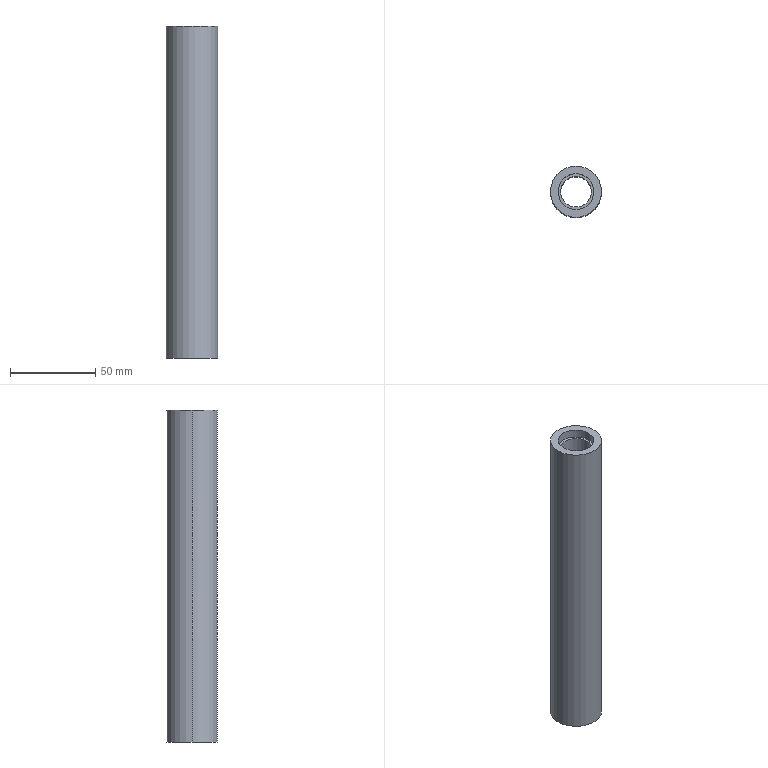Part | STEP file | MT-COMBO-119-S042 | 1 solid | 12 faces | box 30 x 30 x 195 mm | volume 87297 mm3 | cylinder 8 | plane 4 | commonest cylinder face diameters 21 x4 18 x2 30 x2
STEP:
#1=CARTESIAN_POINT('',(-9.,0.,190.));
#2=VERTEX_POINT('',#1);
#3=CARTESIAN_POINT('',(9.,0.,190.));
#4=VERTEX_POINT('',#3);
#5=CARTESIAN_POINT('',(0.,0.,190.));
#6=DIRECTION('',(0.,0.,1.));
#7=DIRECTION('',(1.,0.,0.));
#8=AXIS2_PLACEMENT_3D('',#5,#6,#7);
#9=CIRCLE('',#8,9.);
#10=EDGE_CURVE('',#2,#4,#9,.T.);
#11=ORIENTED_EDGE('',*,*,#10,.T.);
#12=CARTESIAN_POINT('',(9.,0.,5.));
#13=VERTEX_POINT('',#12);
#14=CARTESIAN_POINT('',(9.,0.,195.));
#15=DIRECTION('',(0.,0.,-1.));
#16=VECTOR('',#15,1000.);
#17=LINE('',#14,#16);
#18=EDGE_CURVE('',#4,#13,#17,.T.);
#19=ORIENTED_EDGE('',*,*,#18,.T.);
#20=CARTESIAN_POINT('',(-9.,0.,5.));
#21=VERTEX_POINT('',#20);
#22=CARTESIAN_POINT('',(0.,0.,5.));
#23=DIRECTION('',(0.,0.,-1.));
#24=DIRECTION('',(-1.,0.,0.));
#25=AXIS2_PLACEMENT_3D('',#22,#23,#24);
#26=CIRCLE('',#25,9.);
#27=EDGE_CURVE('',#13,#21,#26,.T.);
#28=ORIENTED_EDGE('',*,*,#27,.T.);
#29=CARTESIAN_POINT('',(-9.,0.,195.));
#30=DIRECTION('',(0.,0.,-1.));
#31=VECTOR('',#30,1000.);
#32=LINE('',#29,#31);
#33=EDGE_CURVE('',#2,#21,#32,.T.);
#34=ORIENTED_EDGE('',*,*,#33,.F.);
#35=EDGE_LOOP('',(#11,#19,#28,#34));
#36=FACE_OUTER_BOUND('',#35,.T.);
#37=CARTESIAN_POINT('',(0.,0.,195.));
#38=DIRECTION('',(0.,0.,-1.));
#39=DIRECTION('',(-1.,0.,0.));
#40=AXIS2_PLACEMENT_3D('',#37,#38,#39);
#41=CYLINDRICAL_SURFACE('',#40,9.);
#42=ADVANCED_FACE('',(#36),#41,.F.);
#43=CARTESIAN_POINT('',(10.5,0.,5.));
#44=VERTEX_POINT('',#43);
#45=CARTESIAN_POINT('',(-10.5,0.,5.));
#46=VERTEX_POINT('',#45);
#47=CARTESIAN_POINT('',(0.,0.,5.));
#48=DIRECTION('',(0.,0.,-1.));
#49=DIRECTION('',(-1.,0.,0.));
#50=AXIS2_PLACEMENT_3D('',#47,#48,#49);
#51=CIRCLE('',#50,10.5);
#52=EDGE_CURVE('',#44,#46,#51,.T.);
#53=ORIENTED_EDGE('',*,*,#52,.F.);
#54=CARTESIAN_POINT('',(10.5,0.,0.));
#55=VERTEX_POINT('',#54);
#56=CARTESIAN_POINT('',(10.5,0.,5.));
#57=DIRECTION('',(0.,0.,-1.));
#58=VECTOR('',#57,1000.);
#59=LINE('',#56,#58);
#60=EDGE_CURVE('',#44,#55,#59,.T.);
#61=ORIENTED_EDGE('',*,*,#60,.T.);
#62=CARTESIAN_POINT('',(-10.5,0.,0.));
#63=VERTEX_POINT('',#62);
#64=CARTESIAN_POINT('',(0.,0.,0.));
#65=DIRECTION('',(0.,0.,-1.));
#66=DIRECTION('',(-1.,0.,0.));
#67=AXIS2_PLACEMENT_3D('',#64,#65,#66);
#68=CIRCLE('',#67,10.5);
#69=EDGE_CURVE('',#55,#63,#68,.T.);
#70=ORIENTED_EDGE('',*,*,#69,.T.);
#71=CARTESIAN_POINT('',(-10.5,0.,5.));
#72=DIRECTION('',(0.,0.,-1.));
#73=VECTOR('',#72,1000.);
#74=LINE('',#71,#73);
#75=EDGE_CURVE('',#46,#63,#74,.T.);
#76=ORIENTED_EDGE('',*,*,#75,.F.);
#77=EDGE_LOOP('',(#53,#61,#70,#76));
#78=FACE_OUTER_BOUND('',#77,.T.);
#79=CARTESIAN_POINT('',(0.,0.,5.));
#80=DIRECTION('',(0.,0.,-1.));
#81=DIRECTION('',(-1.,0.,0.));
#82=AXIS2_PLACEMENT_3D('',#79,#80,#81);
#83=CYLINDRICAL_SURFACE('',#82,10.5);
#84=ADVANCED_FACE('',(#78),#83,.F.);
#85=CARTESIAN_POINT('',(-10.5,0.,190.));
#86=VERTEX_POINT('',#85);
#87=CARTESIAN_POINT('',(10.5,0.,190.));
#88=VERTEX_POINT('',#87);
#89=CARTESIAN_POINT('',(0.,0.,190.));
#90=DIRECTION('',(0.,0.,1.));
#91=DIRECTION('',(1.,0.,0.));
#92=AXIS2_PLACEMENT_3D('',#89,#90,#91);
#93=CIRCLE('',#92,10.5);
#94=EDGE_CURVE('',#86,#88,#93,.T.);
#95=ORIENTED_EDGE('',*,*,#94,.F.);
#96=CARTESIAN_POINT('',(-10.5,0.,195.));
#97=VERTEX_POINT('',#96);
#98=CARTESIAN_POINT('',(-10.5,0.,190.));
#99=DIRECTION('',(0.,0.,1.));
#100=VECTOR('',#99,1000.);
#101=LINE('',#98,#100);
#102=EDGE_CURVE('',#86,#97,#101,.T.);
#103=ORIENTED_EDGE('',*,*,#102,.T.);
#104=CARTESIAN_POINT('',(10.5,0.,195.));
#105=VERTEX_POINT('',#104);
#106=CARTESIAN_POINT('',(0.,0.,195.));
#107=DIRECTION('',(0.,0.,1.));
#108=DIRECTION('',(1.,0.,0.));
#109=AXIS2_PLACEMENT_3D('',#106,#107,#108);
#110=CIRCLE('',#109,10.5);
#111=EDGE_CURVE('',#97,#105,#110,.T.);
#112=ORIENTED_EDGE('',*,*,#111,.T.);
#113=CARTESIAN_POINT('',(10.5,0.,190.));
#114=DIRECTION('',(0.,0.,1.));
#115=VECTOR('',#114,1000.);
#116=LINE('',#113,#115);
#117=EDGE_CURVE('',#88,#105,#116,.T.);
#118=ORIENTED_EDGE('',*,*,#117,.F.);
#119=EDGE_LOOP('',(#95,#103,#112,#118));
#120=FACE_OUTER_BOUND('',#119,.T.);
#121=CARTESIAN_POINT('',(0.,0.,190.));
#122=DIRECTION('',(0.,0.,1.));
#123=DIRECTION('',(1.,0.,0.));
#124=AXIS2_PLACEMENT_3D('',#121,#122,#123);
#125=CYLINDRICAL_SURFACE('',#124,10.5);
#126=ADVANCED_FACE('',(#120),#125,.F.);
#127=CARTESIAN_POINT('',(15.,0.,195.));
#128=VERTEX_POINT('',#127);
#129=CARTESIAN_POINT('',(-15.,0.,195.));
#130=VERTEX_POINT('',#129);
#131=CARTESIAN_POINT('',(0.,0.,195.));
#132=DIRECTION('',(0.,0.,1.));
#133=DIRECTION('',(1.,0.,0.));
#134=AXIS2_PLACEMENT_3D('',#131,#132,#133);
#135=CIRCLE('',#134,15.);
#136=EDGE_CURVE('',#128,#130,#135,.T.);
#137=ORIENTED_EDGE('',*,*,#136,.F.);
#138=CARTESIAN_POINT('',(15.,0.,0.));
#139=VERTEX_POINT('',#138);
#140=CARTESIAN_POINT('',(15.,0.,195.));
#141=DIRECTION('',(0.,0.,-1.));
#142=VECTOR('',#141,1000.);
#143=LINE('',#140,#142);
#144=EDGE_CURVE('',#128,#139,#143,.T.);
#145=ORIENTED_EDGE('',*,*,#144,.T.);
#146=CARTESIAN_POINT('',(-15.,0.,0.));
#147=VERTEX_POINT('',#146);
#148=CARTESIAN_POINT('',(0.,0.,0.));
#149=DIRECTION('',(0.,0.,1.));
#150=DIRECTION('',(1.,0.,0.));
#151=AXIS2_PLACEMENT_3D('',#148,#149,#150);
#152=CIRCLE('',#151,15.);
#153=EDGE_CURVE('',#139,#147,#152,.T.);
#154=ORIENTED_EDGE('',*,*,#153,.T.);
#155=CARTESIAN_POINT('',(-15.,0.,195.));
#156=DIRECTION('',(0.,0.,-1.));
#157=VECTOR('',#156,1000.);
#158=LINE('',#155,#157);
#159=EDGE_CURVE('',#130,#147,#158,.T.);
#160=ORIENTED_EDGE('',*,*,#159,.F.);
#161=EDGE_LOOP('',(#137,#145,#154,#160));
#162=FACE_OUTER_BOUND('',#161,.T.);
#163=CARTESIAN_POINT('',(0.,0.,195.));
#164=DIRECTION('',(0.,0.,-1.));
#165=DIRECTION('',(-1.,0.,0.));
#166=AXIS2_PLACEMENT_3D('',#163,#164,#165);
#167=CYLINDRICAL_SURFACE('',#166,15.);
#168=ADVANCED_FACE('',(#162),#167,.T.);
#169=ORIENTED_EDGE('',*,*,#144,.F.);
#170=CARTESIAN_POINT('',(0.,0.,195.));
#171=DIRECTION('',(0.,0.,1.));
#172=DIRECTION('',(1.,0.,0.));
#173=AXIS2_PLACEMENT_3D('',#170,#171,#172);
#174=CIRCLE('',#173,15.);
#175=EDGE_CURVE('',#130,#128,#174,.T.);
#176=ORIENTED_EDGE('',*,*,#175,.F.);
#177=ORIENTED_EDGE('',*,*,#159,.T.);
#178=CARTESIAN_POINT('',(0.,0.,0.));
#179=DIRECTION('',(0.,0.,1.));
#180=DIRECTION('',(1.,0.,0.));
#181=AXIS2_PLACEMENT_3D('',#178,#179,#180);
#182=CIRCLE('',#181,15.);
#183=EDGE_CURVE('',#147,#139,#182,.T.);
#184=ORIENTED_EDGE('',*,*,#183,.T.);
#185=EDGE_LOOP('',(#169,#176,#177,#184));
#186=FACE_OUTER_BOUND('',#185,.T.);
#187=CARTESIAN_POINT('',(0.,0.,195.));
#188=DIRECTION('',(0.,0.,-1.));
#189=DIRECTION('',(-1.,0.,0.));
#190=AXIS2_PLACEMENT_3D('',#187,#188,#189);
#191=CYLINDRICAL_SURFACE('',#190,15.);
#192=ADVANCED_FACE('',(#186),#191,.T.);
#193=CARTESIAN_POINT('',(0.,0.,195.));
#194=DIRECTION('',(0.,0.,1.));
#195=DIRECTION('',(1.,0.,0.));
#196=AXIS2_PLACEMENT_3D('',#193,#194,#195);
#197=CIRCLE('',#196,10.5);
#198=EDGE_CURVE('',#105,#97,#197,.T.);
#199=ORIENTED_EDGE('',*,*,#198,.F.);
#200=ORIENTED_EDGE('',*,*,#111,.F.);
#201=EDGE_LOOP('',(#199,#200));
#202=FACE_BOUND('',#201,.T.);
#203=ORIENTED_EDGE('',*,*,#175,.T.);
#204=ORIENTED_EDGE('',*,*,#136,.T.);
#205=EDGE_LOOP('',(#203,#204));
#206=FACE_OUTER_BOUND('',#205,.T.);
#207=CARTESIAN_POINT('',(0.,0.,195.));
#208=DIRECTION('',(0.,0.,1.));
#209=DIRECTION('',(1.,0.,0.));
#210=AXIS2_PLACEMENT_3D('',#207,#208,#209);
#211=PLANE('',#210);
#212=ADVANCED_FACE('',(#202,#206),#211,.T.);
#213=CARTESIAN_POINT('',(0.,0.,0.));
#214=DIRECTION('',(0.,0.,-1.));
#215=DIRECTION('',(-1.,0.,0.));
#216=AXIS2_PLACEMENT_3D('',#213,#214,#215);
#217=CIRCLE('',#216,10.5);
#218=EDGE_CURVE('',#63,#55,#217,.T.);
#219=ORIENTED_EDGE('',*,*,#218,.F.);
#220=ORIENTED_EDGE('',*,*,#69,.F.);
#221=EDGE_LOOP('',(#219,#220));
#222=FACE_BOUND('',#221,.T.);
#223=ORIENTED_EDGE('',*,*,#183,.F.);
#224=ORIENTED_EDGE('',*,*,#153,.F.);
#225=EDGE_LOOP('',(#223,#224));
#226=FACE_OUTER_BOUND('',#225,.T.);
#227=CARTESIAN_POINT('',(0.,0.,0.));
#228=DIRECTION('',(0.,0.,1.));
#229=DIRECTION('',(1.,0.,0.));
#230=AXIS2_PLACEMENT_3D('',#227,#228,#229);
#231=PLANE('',#230);
#232=ADVANCED_FACE('',(#222,#226),#231,.F.);
#233=ORIENTED_EDGE('',*,*,#102,.F.);
#234=CARTESIAN_POINT('',(0.,0.,190.));
#235=DIRECTION('',(0.,0.,1.));
#236=DIRECTION('',(1.,0.,0.));
#237=AXIS2_PLACEMENT_3D('',#234,#235,#236);
#238=CIRCLE('',#237,10.5);
#239=EDGE_CURVE('',#88,#86,#238,.T.);
#240=ORIENTED_EDGE('',*,*,#239,.F.);
#241=ORIENTED_EDGE('',*,*,#117,.T.);
#242=ORIENTED_EDGE('',*,*,#198,.T.);
#243=EDGE_LOOP('',(#233,#240,#241,#242));
#244=FACE_OUTER_BOUND('',#243,.T.);
#245=CARTESIAN_POINT('',(0.,0.,190.));
#246=DIRECTION('',(0.,0.,1.));
#247=DIRECTION('',(1.,0.,0.));
#248=AXIS2_PLACEMENT_3D('',#245,#246,#247);
#249=CYLINDRICAL_SURFACE('',#248,10.5);
#250=ADVANCED_FACE('',(#244),#249,.F.);
#251=ORIENTED_EDGE('',*,*,#10,.F.);
#252=CARTESIAN_POINT('',(0.,0.,190.));
#253=DIRECTION('',(0.,0.,1.));
#254=DIRECTION('',(1.,0.,0.));
#255=AXIS2_PLACEMENT_3D('',#252,#253,#254);
#256=CIRCLE('',#255,9.);
#257=EDGE_CURVE('',#4,#2,#256,.T.);
#258=ORIENTED_EDGE('',*,*,#257,.F.);
#259=EDGE_LOOP('',(#251,#258));
#260=FACE_BOUND('',#259,.T.);
#261=ORIENTED_EDGE('',*,*,#239,.T.);
#262=ORIENTED_EDGE('',*,*,#94,.T.);
#263=EDGE_LOOP('',(#261,#262));
#264=FACE_OUTER_BOUND('',#263,.T.);
#265=CARTESIAN_POINT('',(0.,0.,190.));
#266=DIRECTION('',(0.,0.,1.));
#267=DIRECTION('',(1.,0.,0.));
#268=AXIS2_PLACEMENT_3D('',#265,#266,#267);
#269=PLANE('',#268);
#270=ADVANCED_FACE('',(#260,#264),#269,.T.);
#271=ORIENTED_EDGE('',*,*,#60,.F.);
#272=CARTESIAN_POINT('',(0.,0.,5.));
#273=DIRECTION('',(0.,0.,-1.));
#274=DIRECTION('',(-1.,0.,0.));
#275=AXIS2_PLACEMENT_3D('',#272,#273,#274);
#276=CIRCLE('',#275,10.5);
#277=EDGE_CURVE('',#46,#44,#276,.T.);
#278=ORIENTED_EDGE('',*,*,#277,.F.);
#279=ORIENTED_EDGE('',*,*,#75,.T.);
#280=ORIENTED_EDGE('',*,*,#218,.T.);
#281=EDGE_LOOP('',(#271,#278,#279,#280));
#282=FACE_OUTER_BOUND('',#281,.T.);
#283=CARTESIAN_POINT('',(0.,0.,5.));
#284=DIRECTION('',(0.,0.,-1.));
#285=DIRECTION('',(-1.,0.,0.));
#286=AXIS2_PLACEMENT_3D('',#283,#284,#285);
#287=CYLINDRICAL_SURFACE('',#286,10.5);
#288=ADVANCED_FACE('',(#282),#287,.F.);
#289=CARTESIAN_POINT('',(0.,0.,5.));
#290=DIRECTION('',(0.,0.,-1.));
#291=DIRECTION('',(-1.,0.,0.));
#292=AXIS2_PLACEMENT_3D('',#289,#290,#291);
#293=CIRCLE('',#292,9.);
#294=EDGE_CURVE('',#21,#13,#293,.T.);
#295=ORIENTED_EDGE('',*,*,#294,.F.);
#296=ORIENTED_EDGE('',*,*,#27,.F.);
#297=EDGE_LOOP('',(#295,#296));
#298=FACE_BOUND('',#297,.T.);
#299=ORIENTED_EDGE('',*,*,#277,.T.);
#300=ORIENTED_EDGE('',*,*,#52,.T.);
#301=EDGE_LOOP('',(#299,#300));
#302=FACE_OUTER_BOUND('',#301,.T.);
#303=CARTESIAN_POINT('',(0.,0.,5.));
#304=DIRECTION('',(0.,0.,-1.));
#305=DIRECTION('',(-1.,0.,0.));
#306=AXIS2_PLACEMENT_3D('',#303,#304,#305);
#307=PLANE('',#306);
#308=ADVANCED_FACE('',(#298,#302),#307,.T.);
#309=ORIENTED_EDGE('',*,*,#18,.F.);
#310=ORIENTED_EDGE('',*,*,#257,.T.);
#311=ORIENTED_EDGE('',*,*,#33,.T.);
#312=ORIENTED_EDGE('',*,*,#294,.T.);
#313=EDGE_LOOP('',(#309,#310,#311,#312));
#314=FACE_OUTER_BOUND('',#313,.T.);
#315=CARTESIAN_POINT('',(0.,0.,195.));
#316=DIRECTION('',(0.,0.,-1.));
#317=DIRECTION('',(-1.,0.,0.));
#318=AXIS2_PLACEMENT_3D('',#315,#316,#317);
#319=CYLINDRICAL_SURFACE('',#318,9.);
#320=ADVANCED_FACE('',(#314),#319,.F.);
#321=CLOSED_SHELL('',(#42,#84,#126,#168,#192,#212,#232,#250,#270,#288,#308,#320));
#322=MANIFOLD_SOLID_BREP('',#321);
#323=CARTESIAN_POINT('',(0.,0.,0.));
#324=DIRECTION('',(0.,0.,1.));
#325=DIRECTION('',(1.,0.,0.));
#326=AXIS2_PLACEMENT_3D('',#323,#324,#325);
#327=(LENGTH_UNIT()NAMED_UNIT(*)SI_UNIT(.MILLI.,.METRE.));
#328=UNCERTAINTY_MEASURE_WITH_UNIT(LENGTH_MEASURE(0.00001),#327,'','');
#329=(NAMED_UNIT(*)PLANE_ANGLE_UNIT()SI_UNIT($,.RADIAN.));
#330=(NAMED_UNIT(*)SI_UNIT($,.STERADIAN.)SOLID_ANGLE_UNIT());
#331=(GEOMETRIC_REPRESENTATION_CONTEXT(3)GLOBAL_UNCERTAINTY_ASSIGNED_CONTEXT((#328))GLOBAL_UNIT_ASSIGNED_CONTEXT((#327,#329,#330))REPRESENTATION_CONTEXT('',''));
#332=ADVANCED_BREP_SHAPE_REPRESENTATION('',(#322,#326),#331);